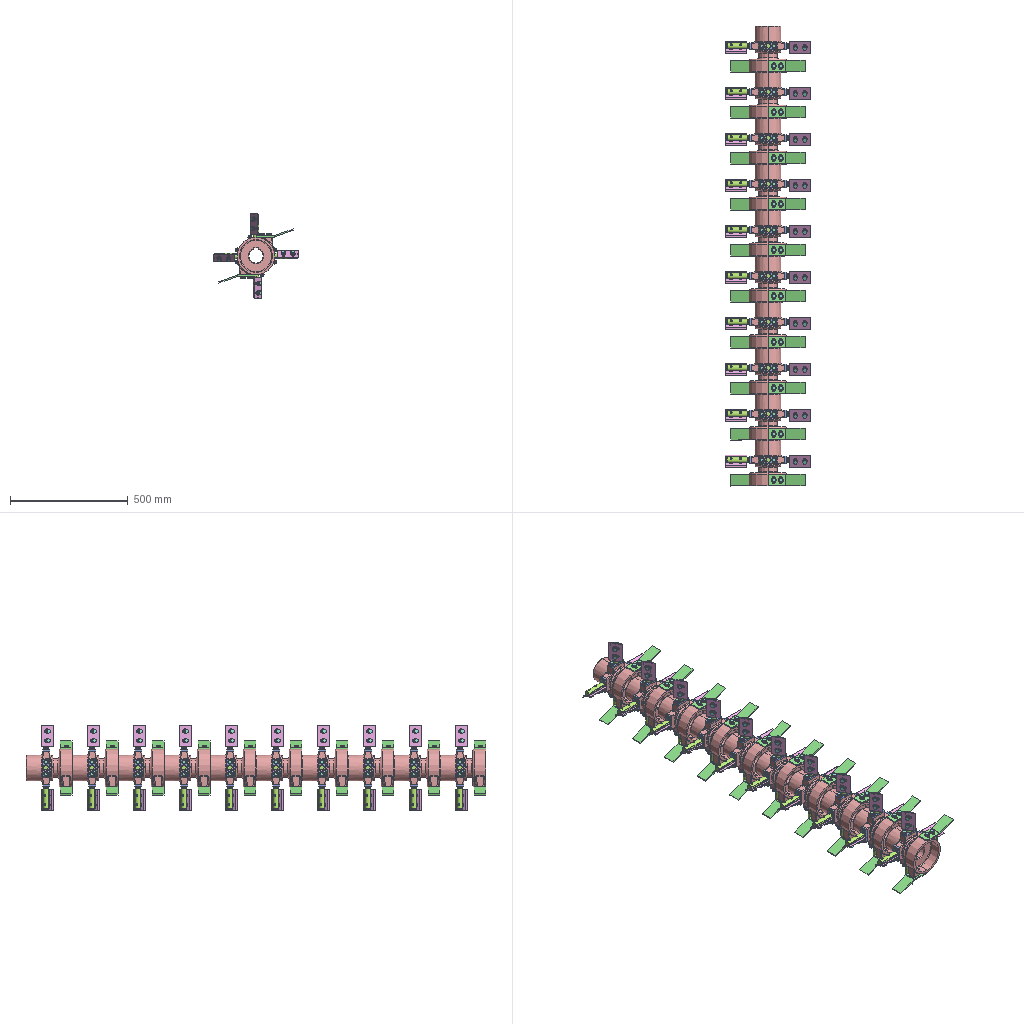Assembly | SolidWorks | 9 different items | 790 placed | box 362 x 1950 x 362 mm
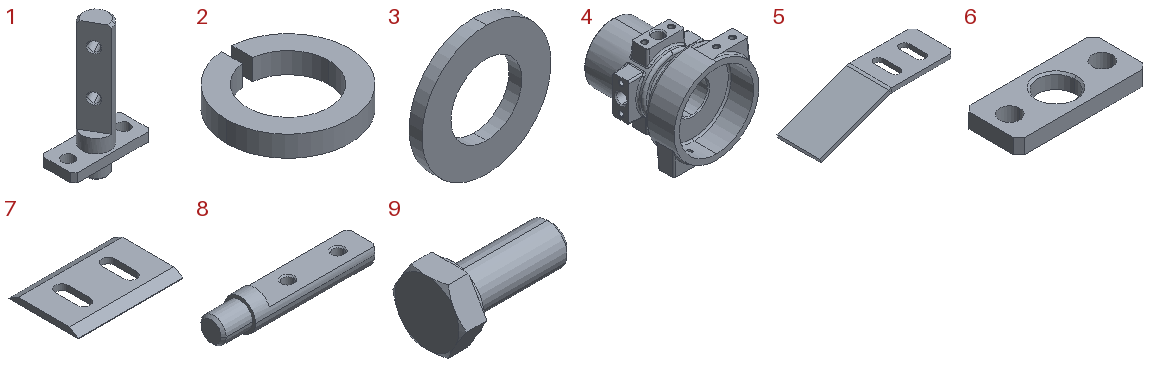Parts list (item | name | quantity | parent item | size | volume | features):
1 | (subassembly) | x40 | - | 70 x 30 x 120 mm | 54696 mm3 | features AEMSimFeature 1
2 | - | x200 | - | 15.372 x 15.344 x 2.6 mm | 261.313 mm3 | features Extrusion 1
3 | - | x200 | - | 20 x 2 x 20 mm | 438.252 mm3 | features Revolution 1
4 | - | x10 | - | 160 x 195 x 160 mm | 950128 mm3 | features ICE 9, Chamfer 8, CirPattern 5, Fillet 3, HoleWzd 2, Revolution 1
5 | - | x20 | - | 158.693 x 50 x 34.796 mm | 37608 mm3 | features Chamfer 1, FlatPattern 1, ICE 1, SMBaseFlange 1, SheetMetal 1
6 | - | x40 | in 1 | 70 x 30 x 8 mm | 12590 mm3 | features Chamfer 2, FlatPattern 1, ICE 1, SMBaseFlange 1, SheetMetal 1
7 | - | x40 | - | 90 x 60 x 5 mm | 20803 mm3 | features Chamfer 2, FlatPattern 1, SMBaseFlange 1, SheetMetal 1
8 | - | x40 | in 1 | 120 x 25 x 25 mm | 42106 mm3 | features Chamfer 2, HoleWzd 1, ICE 1, Revolution 1
9 | - | x200 | - | 31.4 x 18.475 x 16 mm | 3346 mm3 | features RevCut 4, Chamfer 1, Extrusion 1, Fillet 1, LPattern 1, Revolution 1
Mates (type | each side: item.copy, entity, surface, feature):
In the top assembly
Coincident | 4.1 face plane Boss-Extrude 1 | 6.1 face plane Base-Flange 1
Concentric | 4.1 face cylinder CirPattern 5 | 6.1 face cylinder Base-Flange 1 | 2 times
Coincident | 8.1 face plane Cut-Extrude 1 | 7.1 face plane Base-Flange 1
DistanceDim | 7.1 face plane Base-Flange 1 | 8.1 face plane Revolve 2
DistanceDim | 7.1 edge | 6.1 face plane Base-Flange 1
Coincident | 3.1 face plane Base-Revolve | 2.1 face plane Extrude 1
Concentric | 3.1 face cylinder Base-Revolve | 2.1 face cylinder Extrude 1
Concentric | 9.1 face cylinder Boss-Revolve 1 | 3.1 face cylinder Base-Revolve
Coincident | 9.1 face plane Base-Extrude | 2.1 face plane Extrude 1
Coincident | 6.1 face plane Base-Flange 1 | 3.1 face plane Base-Revolve
Concentric | 6.1 face cylinder Base-Flange 1 | 2.1 face cylinder Extrude 1
Coincident | 3.2 face plane Base-Revolve | 2.2 face plane Extrude 1
Concentric | 3.2 face cylinder Base-Revolve | 2.2 face cylinder Extrude 1
Concentric | 9.2 face cylinder Boss-Revolve 1 | 2.2 face cylinder Extrude 1
Coincident | 9.2 face plane Base-Extrude | 2.2 face plane Extrude 1
Coincident | 7.1 face plane Base-Flange 1 | 3.2 face plane Base-Revolve
Concentric | 8.1 face cylinder M10 Tapped Hole 1 | 9.2 face cylinder Boss-Revolve 1
Coincident | 2.3 face plane Extrude 1 | 3.3 face plane Base-Revolve
Concentric | 2.3 face cylinder Extrude 1 | 3.3 face cylinder Base-Revolve
Concentric | 9.3 face cylinder Boss-Revolve 1 | 3.3 face cylinder Base-Revolve
Coincident | 9.3 face plane Base-Extrude | 2.3 face plane Extrude 1
Concentric | 4.1 face cylinder CirPattern 7 | 9.3 face cylinder Boss-Revolve 1
Coincident | 4.1 face plane CirPattern 6 | 5.1 face plane Base-Flange 1
Coincident | 4.1 face plane Revolve 1 | 5.1 face plane Base-Flange 1
DistanceDim | 5.1 face plane Cut-Extrude 1 | 4.1 edge
In subassembly 1
Concentric | 6.2 face cylinder Cut-Extrude 1 | 8.2 face cylinder Revolve 2
Coincident | 6.2 face plane Base-Flange 1 | 8.2 face plane Revolve 2
PlanarAngleDim | 8.2 face plane Cut-Extrude 1 | 6.2 face plane Base-Flange 1